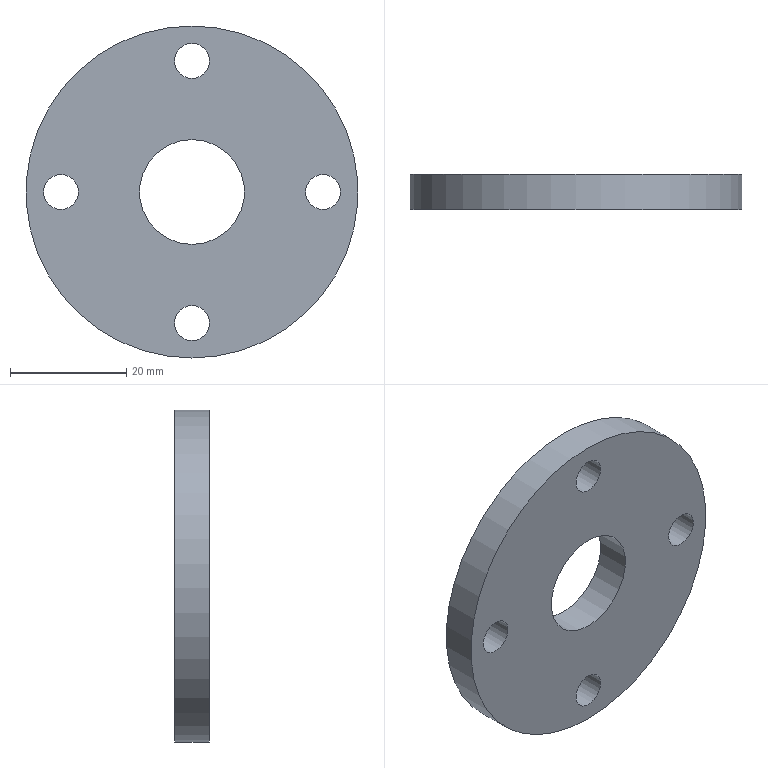Part | STEP file | JBJ-P-1008-05 | 1 solid | 8 faces | box 57 x 6 x 57 mm | volume 13105 mm3 | cylinder 6 | plane 2 | commonest cylinder face diameters 6 x4 18 x1 57 x1
STEP:
#1=CARTESIAN_POINT('',(0.,-6.,28.5));
#2=VERTEX_POINT('',#1);
#3=CARTESIAN_POINT('',(0.,-6.,0.));
#4=DIRECTION('',(0.,1.,0.));
#5=DIRECTION('',(0.,0.,1.));
#6=AXIS2_PLACEMENT_3D('',#3,#4,#5);
#7=CIRCLE('',#6,28.5);
#8=EDGE_CURVE('',#2,#2,#7,.T.);
#9=ORIENTED_EDGE('',*,*,#8,.T.);
#10=EDGE_LOOP('',(#9));
#11=FACE_OUTER_BOUND('',#10,.T.);
#12=CARTESIAN_POINT('',(0.,0.,28.5));
#13=VERTEX_POINT('',#12);
#14=CARTESIAN_POINT('',(0.,0.,0.));
#15=DIRECTION('',(0.,1.,0.));
#16=DIRECTION('',(0.,0.,1.));
#17=AXIS2_PLACEMENT_3D('',#14,#15,#16);
#18=CIRCLE('',#17,28.5);
#19=EDGE_CURVE('',#13,#13,#18,.T.);
#20=ORIENTED_EDGE('',*,*,#19,.F.);
#21=EDGE_LOOP('',(#20));
#22=FACE_OUTER_BOUND('',#21,.T.);
#23=CARTESIAN_POINT('',(0.,-6.,0.));
#24=DIRECTION('',(0.,1.,0.));
#25=DIRECTION('',(0.,0.,1.));
#26=AXIS2_PLACEMENT_3D('',#23,#24,#25);
#27=CYLINDRICAL_SURFACE('',#26,28.5);
#28=ADVANCED_FACE('',(#11,#22),#27,.T.);
#29=CARTESIAN_POINT('',(0.,-6.,9.));
#30=VERTEX_POINT('',#29);
#31=CARTESIAN_POINT('',(0.,-6.,0.));
#32=DIRECTION('',(0.,1.,0.));
#33=DIRECTION('',(0.,0.,1.));
#34=AXIS2_PLACEMENT_3D('',#31,#32,#33);
#35=CIRCLE('',#34,9.);
#36=EDGE_CURVE('',#30,#30,#35,.T.);
#37=ORIENTED_EDGE('',*,*,#36,.T.);
#38=EDGE_LOOP('',(#37));
#39=FACE_BOUND('',#38,.T.);
#40=CARTESIAN_POINT('',(22.5,-6.,3.));
#41=VERTEX_POINT('',#40);
#42=CARTESIAN_POINT('',(22.5,-6.,0.));
#43=DIRECTION('',(0.,1.,0.));
#44=DIRECTION('',(0.,0.,1.));
#45=AXIS2_PLACEMENT_3D('',#42,#43,#44);
#46=CIRCLE('',#45,3.);
#47=EDGE_CURVE('',#41,#41,#46,.T.);
#48=ORIENTED_EDGE('',*,*,#47,.T.);
#49=EDGE_LOOP('',(#48));
#50=FACE_BOUND('',#49,.T.);
#51=CARTESIAN_POINT('',(0.,-6.,25.5));
#52=VERTEX_POINT('',#51);
#53=CARTESIAN_POINT('',(0.,-6.,22.5));
#54=DIRECTION('',(0.,1.,0.));
#55=DIRECTION('',(0.,0.,1.));
#56=AXIS2_PLACEMENT_3D('',#53,#54,#55);
#57=CIRCLE('',#56,3.);
#58=EDGE_CURVE('',#52,#52,#57,.T.);
#59=ORIENTED_EDGE('',*,*,#58,.T.);
#60=EDGE_LOOP('',(#59));
#61=FACE_BOUND('',#60,.T.);
#62=CARTESIAN_POINT('',(0.,-6.,-19.5));
#63=VERTEX_POINT('',#62);
#64=CARTESIAN_POINT('',(0.,-6.,-22.5));
#65=DIRECTION('',(0.,1.,0.));
#66=DIRECTION('',(0.,0.,1.));
#67=AXIS2_PLACEMENT_3D('',#64,#65,#66);
#68=CIRCLE('',#67,3.);
#69=EDGE_CURVE('',#63,#63,#68,.T.);
#70=ORIENTED_EDGE('',*,*,#69,.T.);
#71=EDGE_LOOP('',(#70));
#72=FACE_BOUND('',#71,.T.);
#73=CARTESIAN_POINT('',(-22.5,-6.,3.));
#74=VERTEX_POINT('',#73);
#75=CARTESIAN_POINT('',(-22.5,-6.,0.));
#76=DIRECTION('',(0.,1.,0.));
#77=DIRECTION('',(0.,0.,1.));
#78=AXIS2_PLACEMENT_3D('',#75,#76,#77);
#79=CIRCLE('',#78,3.);
#80=EDGE_CURVE('',#74,#74,#79,.T.);
#81=ORIENTED_EDGE('',*,*,#80,.T.);
#82=EDGE_LOOP('',(#81));
#83=FACE_BOUND('',#82,.T.);
#84=ORIENTED_EDGE('',*,*,#8,.F.);
#85=EDGE_LOOP('',(#84));
#86=FACE_OUTER_BOUND('',#85,.T.);
#87=CARTESIAN_POINT('',(0.,-6.,0.));
#88=DIRECTION('',(0.,1.,0.));
#89=DIRECTION('',(0.,0.,1.));
#90=AXIS2_PLACEMENT_3D('',#87,#88,#89);
#91=PLANE('',#90);
#92=ADVANCED_FACE('',(#39,#50,#61,#72,#83,#86),#91,.F.);
#93=CARTESIAN_POINT('',(0.,0.,9.));
#94=VERTEX_POINT('',#93);
#95=CARTESIAN_POINT('',(0.,0.,0.));
#96=DIRECTION('',(0.,1.,0.));
#97=DIRECTION('',(0.,0.,1.));
#98=AXIS2_PLACEMENT_3D('',#95,#96,#97);
#99=CIRCLE('',#98,9.);
#100=EDGE_CURVE('',#94,#94,#99,.T.);
#101=ORIENTED_EDGE('',*,*,#100,.F.);
#102=EDGE_LOOP('',(#101));
#103=FACE_BOUND('',#102,.T.);
#104=CARTESIAN_POINT('',(22.5,0.,3.));
#105=VERTEX_POINT('',#104);
#106=CARTESIAN_POINT('',(22.5,0.,0.));
#107=DIRECTION('',(0.,1.,0.));
#108=DIRECTION('',(0.,0.,1.));
#109=AXIS2_PLACEMENT_3D('',#106,#107,#108);
#110=CIRCLE('',#109,3.);
#111=EDGE_CURVE('',#105,#105,#110,.T.);
#112=ORIENTED_EDGE('',*,*,#111,.F.);
#113=EDGE_LOOP('',(#112));
#114=FACE_BOUND('',#113,.T.);
#115=CARTESIAN_POINT('',(0.,0.,25.5));
#116=VERTEX_POINT('',#115);
#117=CARTESIAN_POINT('',(0.,0.,22.5));
#118=DIRECTION('',(0.,1.,0.));
#119=DIRECTION('',(0.,0.,1.));
#120=AXIS2_PLACEMENT_3D('',#117,#118,#119);
#121=CIRCLE('',#120,3.);
#122=EDGE_CURVE('',#116,#116,#121,.T.);
#123=ORIENTED_EDGE('',*,*,#122,.F.);
#124=EDGE_LOOP('',(#123));
#125=FACE_BOUND('',#124,.T.);
#126=CARTESIAN_POINT('',(0.,0.,-19.5));
#127=VERTEX_POINT('',#126);
#128=CARTESIAN_POINT('',(0.,0.,-22.5));
#129=DIRECTION('',(0.,1.,0.));
#130=DIRECTION('',(0.,0.,1.));
#131=AXIS2_PLACEMENT_3D('',#128,#129,#130);
#132=CIRCLE('',#131,3.);
#133=EDGE_CURVE('',#127,#127,#132,.T.);
#134=ORIENTED_EDGE('',*,*,#133,.F.);
#135=EDGE_LOOP('',(#134));
#136=FACE_BOUND('',#135,.T.);
#137=CARTESIAN_POINT('',(-22.5,0.,3.));
#138=VERTEX_POINT('',#137);
#139=CARTESIAN_POINT('',(-22.5,0.,0.));
#140=DIRECTION('',(0.,1.,0.));
#141=DIRECTION('',(0.,0.,1.));
#142=AXIS2_PLACEMENT_3D('',#139,#140,#141);
#143=CIRCLE('',#142,3.);
#144=EDGE_CURVE('',#138,#138,#143,.T.);
#145=ORIENTED_EDGE('',*,*,#144,.F.);
#146=EDGE_LOOP('',(#145));
#147=FACE_BOUND('',#146,.T.);
#148=ORIENTED_EDGE('',*,*,#19,.T.);
#149=EDGE_LOOP('',(#148));
#150=FACE_OUTER_BOUND('',#149,.T.);
#151=CARTESIAN_POINT('',(0.,0.,0.));
#152=DIRECTION('',(0.,1.,0.));
#153=DIRECTION('',(0.,0.,1.));
#154=AXIS2_PLACEMENT_3D('',#151,#152,#153);
#155=PLANE('',#154);
#156=ADVANCED_FACE('',(#103,#114,#125,#136,#147,#150),#155,.T.);
#157=ORIENTED_EDGE('',*,*,#80,.F.);
#158=EDGE_LOOP('',(#157));
#159=FACE_OUTER_BOUND('',#158,.T.);
#160=ORIENTED_EDGE('',*,*,#144,.T.);
#161=EDGE_LOOP('',(#160));
#162=FACE_OUTER_BOUND('',#161,.T.);
#163=CARTESIAN_POINT('',(-22.5,-6.,0.));
#164=DIRECTION('',(0.,1.,0.));
#165=DIRECTION('',(0.,0.,1.));
#166=AXIS2_PLACEMENT_3D('',#163,#164,#165);
#167=CYLINDRICAL_SURFACE('',#166,3.);
#168=ADVANCED_FACE('',(#159,#162),#167,.F.);
#169=ORIENTED_EDGE('',*,*,#69,.F.);
#170=EDGE_LOOP('',(#169));
#171=FACE_OUTER_BOUND('',#170,.T.);
#172=ORIENTED_EDGE('',*,*,#133,.T.);
#173=EDGE_LOOP('',(#172));
#174=FACE_OUTER_BOUND('',#173,.T.);
#175=CARTESIAN_POINT('',(0.,-6.,-22.5));
#176=DIRECTION('',(0.,1.,0.));
#177=DIRECTION('',(0.,0.,1.));
#178=AXIS2_PLACEMENT_3D('',#175,#176,#177);
#179=CYLINDRICAL_SURFACE('',#178,3.);
#180=ADVANCED_FACE('',(#171,#174),#179,.F.);
#181=ORIENTED_EDGE('',*,*,#58,.F.);
#182=EDGE_LOOP('',(#181));
#183=FACE_OUTER_BOUND('',#182,.T.);
#184=ORIENTED_EDGE('',*,*,#122,.T.);
#185=EDGE_LOOP('',(#184));
#186=FACE_OUTER_BOUND('',#185,.T.);
#187=CARTESIAN_POINT('',(0.,-6.,22.5));
#188=DIRECTION('',(0.,1.,0.));
#189=DIRECTION('',(0.,0.,1.));
#190=AXIS2_PLACEMENT_3D('',#187,#188,#189);
#191=CYLINDRICAL_SURFACE('',#190,3.);
#192=ADVANCED_FACE('',(#183,#186),#191,.F.);
#193=ORIENTED_EDGE('',*,*,#47,.F.);
#194=EDGE_LOOP('',(#193));
#195=FACE_OUTER_BOUND('',#194,.T.);
#196=ORIENTED_EDGE('',*,*,#111,.T.);
#197=EDGE_LOOP('',(#196));
#198=FACE_OUTER_BOUND('',#197,.T.);
#199=CARTESIAN_POINT('',(22.5,-6.,0.));
#200=DIRECTION('',(0.,1.,0.));
#201=DIRECTION('',(0.,0.,1.));
#202=AXIS2_PLACEMENT_3D('',#199,#200,#201);
#203=CYLINDRICAL_SURFACE('',#202,3.);
#204=ADVANCED_FACE('',(#195,#198),#203,.F.);
#205=ORIENTED_EDGE('',*,*,#100,.T.);
#206=EDGE_LOOP('',(#205));
#207=FACE_OUTER_BOUND('',#206,.T.);
#208=ORIENTED_EDGE('',*,*,#36,.F.);
#209=EDGE_LOOP('',(#208));
#210=FACE_OUTER_BOUND('',#209,.T.);
#211=CARTESIAN_POINT('',(0.,-10.,0.));
#212=DIRECTION('',(0.,1.,0.));
#213=DIRECTION('',(0.,0.,1.));
#214=AXIS2_PLACEMENT_3D('',#211,#212,#213);
#215=CYLINDRICAL_SURFACE('',#214,9.);
#216=ADVANCED_FACE('',(#207,#210),#215,.F.);
#217=CLOSED_SHELL('',(#28,#92,#156,#168,#180,#192,#204,#216));
#218=MANIFOLD_SOLID_BREP('',#217);
#219=CARTESIAN_POINT('',(0.,0.,0.));
#220=DIRECTION('',(0.,0.,1.));
#221=DIRECTION('',(1.,0.,0.));
#222=AXIS2_PLACEMENT_3D('',#219,#220,#221);
#223=(LENGTH_UNIT()NAMED_UNIT(*)SI_UNIT(.MILLI.,.METRE.));
#224=UNCERTAINTY_MEASURE_WITH_UNIT(LENGTH_MEASURE(0.00001),#223,'','');
#225=(NAMED_UNIT(*)PLANE_ANGLE_UNIT()SI_UNIT($,.RADIAN.));
#226=(NAMED_UNIT(*)SI_UNIT($,.STERADIAN.)SOLID_ANGLE_UNIT());
#227=(GEOMETRIC_REPRESENTATION_CONTEXT(3)GLOBAL_UNCERTAINTY_ASSIGNED_CONTEXT((#224))GLOBAL_UNIT_ASSIGNED_CONTEXT((#223,#225,#226))REPRESENTATION_CONTEXT('',''));
#228=ADVANCED_BREP_SHAPE_REPRESENTATION('',(#218,#222),#227);